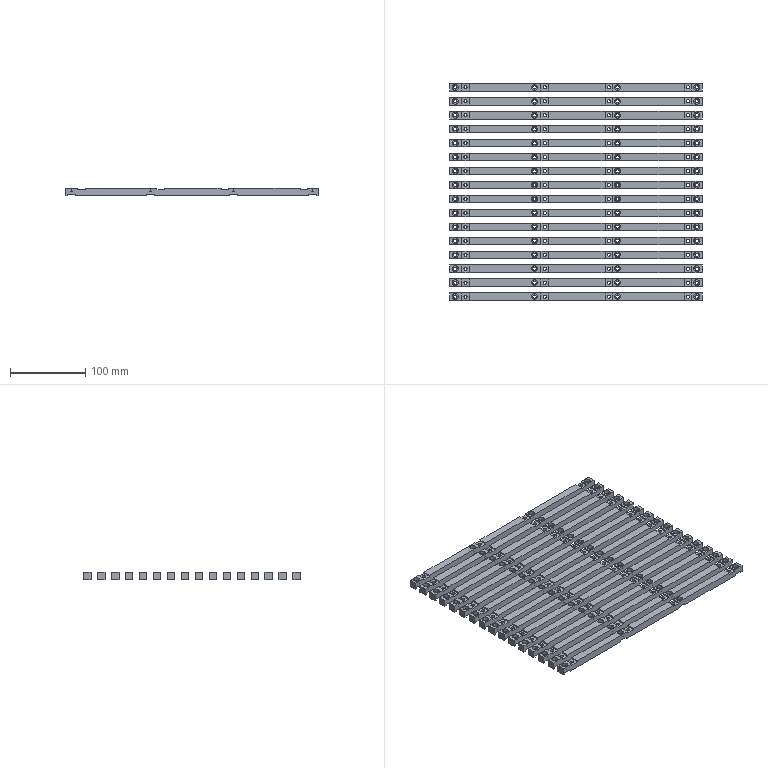Part | 16 solids | 1056 faces | box 335 x 287.5 x 10 mm | volume 485487 mm3 | plane 672 | cylinder 384 | commonest cylinder face diameters 4.2 x128 4.5 x128 8 x128